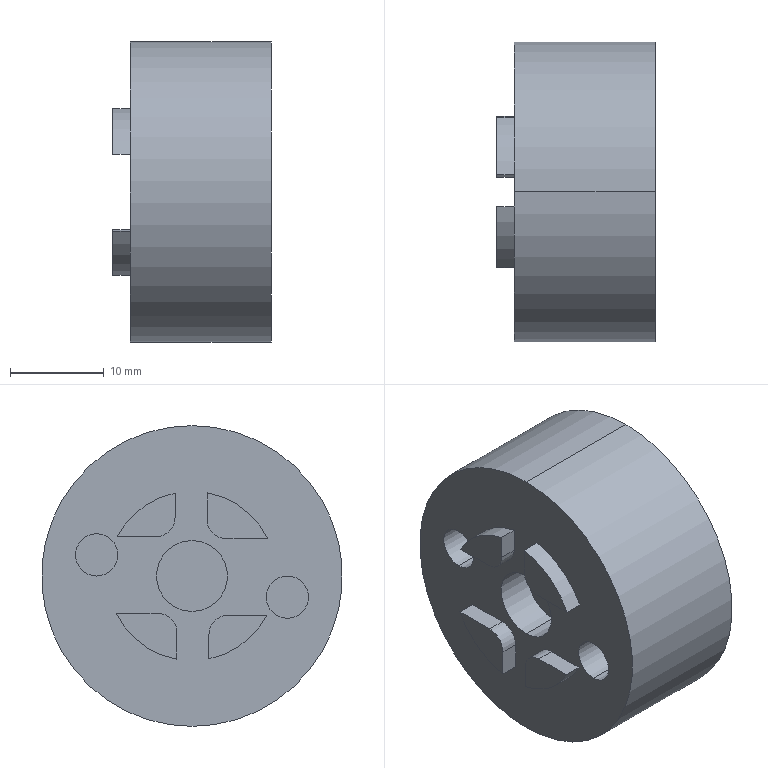Part | SolidWorks | features ICE 6, Cut 1, Extrusion 1, Fillet 1 | 1 solid | 38 faces | box 16.9 x 32 x 32 mm | volume 11867 mm3 | plane 22 | cylinder 16 | commonest cylinder face diameters 4 x4 4.5 x4 18 x4 7.55 x2 32 x2
STEP:
#1=CARTESIAN_POINT('',(3.5,-10.15,-4.5));
#2=VERTEX_POINT('',#1);
#3=CARTESIAN_POINT('',(3.5,-10.15,0.));
#4=VERTEX_POINT('',#3);
#5=CARTESIAN_POINT('',(3.5,-10.15,-2.25));
#6=DIRECTION('',(-1.,0.,0.));
#7=DIRECTION('',(0.,0.,1.));
#8=AXIS2_PLACEMENT_3D('',#5,#6,#7);
#9=CIRCLE('',#8,2.25);
#10=EDGE_CURVE('',#2,#4,#9,.T.);
#11=ORIENTED_EDGE('',*,*,#10,.F.);
#12=CARTESIAN_POINT('',(0.,-10.15,-4.5));
#13=VERTEX_POINT('',#12);
#14=CARTESIAN_POINT('',(3.5,-10.15,-4.5));
#15=DIRECTION('',(-1.,0.,0.));
#16=VECTOR('',#15,1000.);
#17=LINE('',#14,#16);
#18=EDGE_CURVE('',#2,#13,#17,.T.);
#19=ORIENTED_EDGE('',*,*,#18,.T.);
#20=CARTESIAN_POINT('',(0.,-10.15,0.));
#21=VERTEX_POINT('',#20);
#22=CARTESIAN_POINT('',(0.,-10.15,-2.25));
#23=DIRECTION('',(-1.,0.,0.));
#24=DIRECTION('',(0.,0.,1.));
#25=AXIS2_PLACEMENT_3D('',#22,#23,#24);
#26=CIRCLE('',#25,2.25);
#27=EDGE_CURVE('',#13,#21,#26,.T.);
#28=ORIENTED_EDGE('',*,*,#27,.T.);
#29=CARTESIAN_POINT('',(3.5,-10.15,0.));
#30=DIRECTION('',(-1.,0.,0.));
#31=VECTOR('',#30,1000.);
#32=LINE('',#29,#31);
#33=EDGE_CURVE('',#4,#21,#32,.T.);
#34=ORIENTED_EDGE('',*,*,#33,.F.);
#35=EDGE_LOOP('',(#11,#19,#28,#34));
#36=FACE_OUTER_BOUND('',#35,.T.);
#37=CARTESIAN_POINT('',(3.5,-10.15,-2.25));
#38=DIRECTION('',(-1.,0.,0.));
#39=DIRECTION('',(0.,0.,1.));
#40=AXIS2_PLACEMENT_3D('',#37,#38,#39);
#41=CYLINDRICAL_SURFACE('',#40,2.25);
#42=ADVANCED_FACE('',(#36),#41,.F.);
#43=CARTESIAN_POINT('',(3.5,10.15,0.));
#44=VERTEX_POINT('',#43);
#45=CARTESIAN_POINT('',(3.5,10.15,4.5));
#46=VERTEX_POINT('',#45);
#47=CARTESIAN_POINT('',(3.5,10.15,2.25));
#48=DIRECTION('',(-1.,0.,0.));
#49=DIRECTION('',(0.,0.,1.));
#50=AXIS2_PLACEMENT_3D('',#47,#48,#49);
#51=CIRCLE('',#50,2.25);
#52=EDGE_CURVE('',#44,#46,#51,.T.);
#53=ORIENTED_EDGE('',*,*,#52,.F.);
#54=CARTESIAN_POINT('',(0.,10.15,0.));
#55=VERTEX_POINT('',#54);
#56=CARTESIAN_POINT('',(3.5,10.15,0.));
#57=DIRECTION('',(-1.,0.,0.));
#58=VECTOR('',#57,1000.);
#59=LINE('',#56,#58);
#60=EDGE_CURVE('',#44,#55,#59,.T.);
#61=ORIENTED_EDGE('',*,*,#60,.T.);
#62=CARTESIAN_POINT('',(0.,10.15,4.5));
#63=VERTEX_POINT('',#62);
#64=CARTESIAN_POINT('',(0.,10.15,2.25));
#65=DIRECTION('',(-1.,0.,0.));
#66=DIRECTION('',(0.,0.,1.));
#67=AXIS2_PLACEMENT_3D('',#64,#65,#66);
#68=CIRCLE('',#67,2.25);
#69=EDGE_CURVE('',#55,#63,#68,.T.);
#70=ORIENTED_EDGE('',*,*,#69,.T.);
#71=CARTESIAN_POINT('',(3.5,10.15,4.5));
#72=DIRECTION('',(-1.,0.,0.));
#73=VECTOR('',#72,1000.);
#74=LINE('',#71,#73);
#75=EDGE_CURVE('',#46,#63,#74,.T.);
#76=ORIENTED_EDGE('',*,*,#75,.F.);
#77=EDGE_LOOP('',(#53,#61,#70,#76));
#78=FACE_OUTER_BOUND('',#77,.T.);
#79=CARTESIAN_POINT('',(3.5,10.15,2.25));
#80=DIRECTION('',(-1.,0.,0.));
#81=DIRECTION('',(0.,0.,1.));
#82=AXIS2_PLACEMENT_3D('',#79,#80,#81);
#83=CYLINDRICAL_SURFACE('',#82,2.25);
#84=ADVANCED_FACE('',(#78),#83,.F.);
#85=CARTESIAN_POINT('',(4.,0.,-3.775));
#86=VERTEX_POINT('',#85);
#87=CARTESIAN_POINT('',(4.,0.,3.775));
#88=VERTEX_POINT('',#87);
#89=CARTESIAN_POINT('',(4.,0.,0.));
#90=DIRECTION('',(-1.,0.,0.));
#91=DIRECTION('',(0.,0.,1.));
#92=AXIS2_PLACEMENT_3D('',#89,#90,#91);
#93=CIRCLE('',#92,3.775);
#94=EDGE_CURVE('',#86,#88,#93,.T.);
#95=ORIENTED_EDGE('',*,*,#94,.F.);
#96=CARTESIAN_POINT('',(0.,0.,-3.775));
#97=VERTEX_POINT('',#96);
#98=CARTESIAN_POINT('',(4.,0.,-3.775));
#99=DIRECTION('',(-1.,0.,0.));
#100=VECTOR('',#99,1000.);
#101=LINE('',#98,#100);
#102=EDGE_CURVE('',#86,#97,#101,.T.);
#103=ORIENTED_EDGE('',*,*,#102,.T.);
#104=CARTESIAN_POINT('',(0.,0.,3.775));
#105=VERTEX_POINT('',#104);
#106=CARTESIAN_POINT('',(0.,0.,0.));
#107=DIRECTION('',(-1.,0.,0.));
#108=DIRECTION('',(0.,0.,1.));
#109=AXIS2_PLACEMENT_3D('',#106,#107,#108);
#110=CIRCLE('',#109,3.775);
#111=EDGE_CURVE('',#97,#105,#110,.T.);
#112=ORIENTED_EDGE('',*,*,#111,.T.);
#113=CARTESIAN_POINT('',(4.,0.,3.775));
#114=DIRECTION('',(-1.,0.,0.));
#115=VECTOR('',#114,1000.);
#116=LINE('',#113,#115);
#117=EDGE_CURVE('',#88,#105,#116,.T.);
#118=ORIENTED_EDGE('',*,*,#117,.F.);
#119=EDGE_LOOP('',(#95,#103,#112,#118));
#120=FACE_OUTER_BOUND('',#119,.T.);
#121=CARTESIAN_POINT('',(4.,0.,0.));
#122=DIRECTION('',(-1.,0.,0.));
#123=DIRECTION('',(0.,0.,1.));
#124=AXIS2_PLACEMENT_3D('',#121,#122,#123);
#125=CYLINDRICAL_SURFACE('',#124,3.775);
#126=ADVANCED_FACE('',(#120),#125,.F.);
#127=CARTESIAN_POINT('',(15.,0.,-16.));
#128=VERTEX_POINT('',#127);
#129=CARTESIAN_POINT('',(15.,0.,16.));
#130=VERTEX_POINT('',#129);
#131=CARTESIAN_POINT('',(15.,0.,0.));
#132=DIRECTION('',(1.,0.,0.));
#133=DIRECTION('',(0.,0.,-1.));
#134=AXIS2_PLACEMENT_3D('',#131,#132,#133);
#135=CIRCLE('',#134,16.);
#136=EDGE_CURVE('',#128,#130,#135,.T.);
#137=ORIENTED_EDGE('',*,*,#136,.F.);
#138=CARTESIAN_POINT('',(0.,0.,-16.));
#139=VERTEX_POINT('',#138);
#140=CARTESIAN_POINT('',(15.,0.,-16.));
#141=DIRECTION('',(-1.,0.,0.));
#142=VECTOR('',#141,1000.);
#143=LINE('',#140,#142);
#144=EDGE_CURVE('',#128,#139,#143,.T.);
#145=ORIENTED_EDGE('',*,*,#144,.T.);
#146=CARTESIAN_POINT('',(0.,0.,16.));
#147=VERTEX_POINT('',#146);
#148=CARTESIAN_POINT('',(0.,0.,0.));
#149=DIRECTION('',(1.,0.,0.));
#150=DIRECTION('',(0.,0.,-1.));
#151=AXIS2_PLACEMENT_3D('',#148,#149,#150);
#152=CIRCLE('',#151,16.);
#153=EDGE_CURVE('',#139,#147,#152,.T.);
#154=ORIENTED_EDGE('',*,*,#153,.T.);
#155=CARTESIAN_POINT('',(15.,0.,16.));
#156=DIRECTION('',(-1.,0.,0.));
#157=VECTOR('',#156,1000.);
#158=LINE('',#155,#157);
#159=EDGE_CURVE('',#130,#147,#158,.T.);
#160=ORIENTED_EDGE('',*,*,#159,.F.);
#161=EDGE_LOOP('',(#137,#145,#154,#160));
#162=FACE_OUTER_BOUND('',#161,.T.);
#163=CARTESIAN_POINT('',(15.,0.,0.));
#164=DIRECTION('',(-1.,0.,0.));
#165=DIRECTION('',(0.,0.,1.));
#166=AXIS2_PLACEMENT_3D('',#163,#164,#165);
#167=CYLINDRICAL_SURFACE('',#166,16.);
#168=ADVANCED_FACE('',(#162),#167,.T.);
#169=CARTESIAN_POINT('',(0.,7.96,4.2));
#170=VERTEX_POINT('',#169);
#171=CARTESIAN_POINT('',(-1.9,7.96,4.2));
#172=VERTEX_POINT('',#171);
#173=CARTESIAN_POINT('',(49.994,7.96,4.2));
#174=DIRECTION('',(-1.,0.,0.));
#175=VECTOR('',#174,1000.);
#176=LINE('',#173,#175);
#177=EDGE_CURVE('',#170,#172,#176,.T.);
#178=ORIENTED_EDGE('',*,*,#177,.F.);
#179=CARTESIAN_POINT('',(0.,3.8,4.2));
#180=VERTEX_POINT('',#179);
#181=CARTESIAN_POINT('',(0.,17.12,4.2));
#182=DIRECTION('',(0.,-1.,0.));
#183=VECTOR('',#182,1000.);
#184=LINE('',#181,#183);
#185=EDGE_CURVE('',#170,#180,#184,.T.);
#186=ORIENTED_EDGE('',*,*,#185,.T.);
#187=CARTESIAN_POINT('',(-1.9,3.8,4.2));
#188=VERTEX_POINT('',#187);
#189=CARTESIAN_POINT('',(-1.9,3.8,4.2));
#190=DIRECTION('',(-1.,0.,0.));
#191=VECTOR('',#190,1000.);
#192=LINE('',#189,#191);
#193=EDGE_CURVE('',#180,#188,#192,.T.);
#194=ORIENTED_EDGE('',*,*,#193,.T.);
#195=CARTESIAN_POINT('',(-1.9,17.12,4.2));
#196=DIRECTION('',(0.,-1.,0.));
#197=VECTOR('',#196,1000.);
#198=LINE('',#195,#197);
#199=EDGE_CURVE('',#172,#188,#198,.T.);
#200=ORIENTED_EDGE('',*,*,#199,.F.);
#201=EDGE_LOOP('',(#178,#186,#194,#200));
#202=FACE_OUTER_BOUND('',#201,.T.);
#203=CARTESIAN_POINT('',(-1.9,17.12,4.2));
#204=DIRECTION('',(0.,0.,1.));
#205=DIRECTION('',(0.,-1.,0.));
#206=AXIS2_PLACEMENT_3D('',#203,#204,#205);
#207=PLANE('',#206);
#208=ADVANCED_FACE('',(#202),#207,.F.);
#209=CARTESIAN_POINT('',(-1.9,1.8,8.818));
#210=VERTEX_POINT('',#209);
#211=CARTESIAN_POINT('',(0.,1.8,8.818));
#212=VERTEX_POINT('',#211);
#213=CARTESIAN_POINT('',(49.994,1.8,8.818));
#214=DIRECTION('',(1.,0.,0.));
#215=VECTOR('',#214,1000.);
#216=LINE('',#213,#215);
#217=EDGE_CURVE('',#210,#212,#216,.T.);
#218=ORIENTED_EDGE('',*,*,#217,.F.);
#219=CARTESIAN_POINT('',(-1.9,1.8,6.2));
#220=VERTEX_POINT('',#219);
#221=CARTESIAN_POINT('',(-1.9,1.8,4.2));
#222=DIRECTION('',(0.,0.,1.));
#223=VECTOR('',#222,1000.);
#224=LINE('',#221,#223);
#225=EDGE_CURVE('',#220,#210,#224,.T.);
#226=ORIENTED_EDGE('',*,*,#225,.F.);
#227=CARTESIAN_POINT('',(0.,1.8,6.2));
#228=VERTEX_POINT('',#227);
#229=CARTESIAN_POINT('',(-1.9,1.8,6.2));
#230=DIRECTION('',(1.,0.,0.));
#231=VECTOR('',#230,1000.);
#232=LINE('',#229,#231);
#233=EDGE_CURVE('',#220,#228,#232,.T.);
#234=ORIENTED_EDGE('',*,*,#233,.T.);
#235=CARTESIAN_POINT('',(0.,1.8,4.2));
#236=DIRECTION('',(0.,0.,1.));
#237=VECTOR('',#236,1000.);
#238=LINE('',#235,#237);
#239=EDGE_CURVE('',#228,#212,#238,.T.);
#240=ORIENTED_EDGE('',*,*,#239,.T.);
#241=EDGE_LOOP('',(#218,#226,#234,#240));
#242=FACE_OUTER_BOUND('',#241,.T.);
#243=CARTESIAN_POINT('',(-1.9,1.8,4.2));
#244=DIRECTION('',(0.,1.,0.));
#245=DIRECTION('',(0.,0.,1.));
#246=AXIS2_PLACEMENT_3D('',#243,#244,#245);
#247=PLANE('',#246);
#248=ADVANCED_FACE('',(#242),#247,.F.);
#249=ORIENTED_EDGE('',*,*,#225,.T.);
#250=CARTESIAN_POINT('',(-1.9,0.,0.));
#251=DIRECTION('',(-1.,0.,0.));
#252=DIRECTION('',(0.,0.,1.));
#253=AXIS2_PLACEMENT_3D('',#250,#251,#252);
#254=CIRCLE('',#253,9.);
#255=EDGE_CURVE('',#210,#172,#254,.T.);
#256=ORIENTED_EDGE('',*,*,#255,.T.);
#257=ORIENTED_EDGE('',*,*,#199,.T.);
#258=CARTESIAN_POINT('',(-1.9,3.8,6.2));
#259=DIRECTION('',(-1.,0.,0.));
#260=DIRECTION('',(0.,0.,1.));
#261=AXIS2_PLACEMENT_3D('',#258,#259,#260);
#262=CIRCLE('',#261,2.);
#263=EDGE_CURVE('',#188,#220,#262,.T.);
#264=ORIENTED_EDGE('',*,*,#263,.T.);
#265=EDGE_LOOP('',(#249,#256,#257,#264));
#266=FACE_OUTER_BOUND('',#265,.T.);
#267=CARTESIAN_POINT('',(-1.9,0.,0.));
#268=DIRECTION('',(-1.,0.,0.));
#269=DIRECTION('',(0.,0.,1.));
#270=AXIS2_PLACEMENT_3D('',#267,#268,#269);
#271=PLANE('',#270);
#272=ADVANCED_FACE('',(#266),#271,.T.);
#273=CARTESIAN_POINT('',(0.,-7.96,-4.2));
#274=VERTEX_POINT('',#273);
#275=CARTESIAN_POINT('',(-1.9,-7.96,-4.2));
#276=VERTEX_POINT('',#275);
#277=CARTESIAN_POINT('',(49.994,-7.96,-4.2));
#278=DIRECTION('',(-1.,0.,0.));
#279=VECTOR('',#278,1000.);
#280=LINE('',#277,#279);
#281=EDGE_CURVE('',#274,#276,#280,.T.);
#282=ORIENTED_EDGE('',*,*,#281,.F.);
#283=CARTESIAN_POINT('',(0.,-3.8,-4.2));
#284=VERTEX_POINT('',#283);
#285=CARTESIAN_POINT('',(0.,-1.8,-4.2));
#286=DIRECTION('',(0.,1.,0.));
#287=VECTOR('',#286,1000.);
#288=LINE('',#285,#287);
#289=EDGE_CURVE('',#274,#284,#288,.T.);
#290=ORIENTED_EDGE('',*,*,#289,.T.);
#291=CARTESIAN_POINT('',(-1.9,-3.8,-4.2));
#292=VERTEX_POINT('',#291);
#293=CARTESIAN_POINT('',(-1.9,-3.8,-4.2));
#294=DIRECTION('',(-1.,0.,0.));
#295=VECTOR('',#294,1000.);
#296=LINE('',#293,#295);
#297=EDGE_CURVE('',#284,#292,#296,.T.);
#298=ORIENTED_EDGE('',*,*,#297,.T.);
#299=CARTESIAN_POINT('',(-1.9,-1.8,-4.2));
#300=DIRECTION('',(0.,1.,0.));
#301=VECTOR('',#300,1000.);
#302=LINE('',#299,#301);
#303=EDGE_CURVE('',#276,#292,#302,.T.);
#304=ORIENTED_EDGE('',*,*,#303,.F.);
#305=EDGE_LOOP('',(#282,#290,#298,#304));
#306=FACE_OUTER_BOUND('',#305,.T.);
#307=CARTESIAN_POINT('',(-1.9,-1.8,-4.2));
#308=DIRECTION('',(0.,0.,-1.));
#309=DIRECTION('',(-1.,0.,0.));
#310=AXIS2_PLACEMENT_3D('',#307,#308,#309);
#311=PLANE('',#310);
#312=ADVANCED_FACE('',(#306),#311,.F.);
#313=CARTESIAN_POINT('',(-1.9,-1.8,-8.818));
#314=VERTEX_POINT('',#313);
#315=CARTESIAN_POINT('',(0.,-1.8,-8.818));
#316=VERTEX_POINT('',#315);
#317=CARTESIAN_POINT('',(49.994,-1.8,-8.818));
#318=DIRECTION('',(1.,0.,0.));
#319=VECTOR('',#318,1000.);
#320=LINE('',#317,#319);
#321=EDGE_CURVE('',#314,#316,#320,.T.);
#322=ORIENTED_EDGE('',*,*,#321,.F.);
#323=CARTESIAN_POINT('',(-1.9,-1.8,-6.2));
#324=VERTEX_POINT('',#323);
#325=CARTESIAN_POINT('',(-1.9,-1.8,-20.455));
#326=DIRECTION('',(0.,0.,-1.));
#327=VECTOR('',#326,1000.);
#328=LINE('',#325,#327);
#329=EDGE_CURVE('',#324,#314,#328,.T.);
#330=ORIENTED_EDGE('',*,*,#329,.F.);
#331=CARTESIAN_POINT('',(0.,-1.8,-6.2));
#332=VERTEX_POINT('',#331);
#333=CARTESIAN_POINT('',(-1.9,-1.8,-6.2));
#334=DIRECTION('',(1.,0.,0.));
#335=VECTOR('',#334,1000.);
#336=LINE('',#333,#335);
#337=EDGE_CURVE('',#324,#332,#336,.T.);
#338=ORIENTED_EDGE('',*,*,#337,.T.);
#339=CARTESIAN_POINT('',(0.,-1.8,-20.455));
#340=DIRECTION('',(0.,0.,-1.));
#341=VECTOR('',#340,1000.);
#342=LINE('',#339,#341);
#343=EDGE_CURVE('',#332,#316,#342,.T.);
#344=ORIENTED_EDGE('',*,*,#343,.T.);
#345=EDGE_LOOP('',(#322,#330,#338,#344));
#346=FACE_OUTER_BOUND('',#345,.T.);
#347=CARTESIAN_POINT('',(-1.9,-1.8,-20.455));
#348=DIRECTION('',(0.,-1.,0.));
#349=DIRECTION('',(0.,0.,-1.));
#350=AXIS2_PLACEMENT_3D('',#347,#348,#349);
#351=PLANE('',#350);
#352=ADVANCED_FACE('',(#346),#351,.F.);
#353=ORIENTED_EDGE('',*,*,#329,.T.);
#354=CARTESIAN_POINT('',(-1.9,0.,0.));
#355=DIRECTION('',(-1.,0.,0.));
#356=DIRECTION('',(0.,0.,1.));
#357=AXIS2_PLACEMENT_3D('',#354,#355,#356);
#358=CIRCLE('',#357,9.);
#359=EDGE_CURVE('',#314,#276,#358,.T.);
#360=ORIENTED_EDGE('',*,*,#359,.T.);
#361=ORIENTED_EDGE('',*,*,#303,.T.);
#362=CARTESIAN_POINT('',(-1.9,-3.8,-6.2));
#363=DIRECTION('',(-1.,0.,0.));
#364=DIRECTION('',(0.,0.,1.));
#365=AXIS2_PLACEMENT_3D('',#362,#363,#364);
#366=CIRCLE('',#365,2.);
#367=EDGE_CURVE('',#292,#324,#366,.T.);
#368=ORIENTED_EDGE('',*,*,#367,.T.);
#369=EDGE_LOOP('',(#353,#360,#361,#368));
#370=FACE_OUTER_BOUND('',#369,.T.);
#371=CARTESIAN_POINT('',(-1.9,0.,0.));
#372=DIRECTION('',(-1.,0.,0.));
#373=DIRECTION('',(0.,0.,1.));
#374=AXIS2_PLACEMENT_3D('',#371,#372,#373);
#375=PLANE('',#374);
#376=ADVANCED_FACE('',(#370),#375,.T.);
#377=CARTESIAN_POINT('',(-1.9,8.062,-4.));
#378=VERTEX_POINT('',#377);
#379=CARTESIAN_POINT('',(0.,8.062,-4.));
#380=VERTEX_POINT('',#379);
#381=CARTESIAN_POINT('',(49.994,8.062,-4.));
#382=DIRECTION('',(1.,0.,0.));
#383=VECTOR('',#382,1000.);
#384=LINE('',#381,#383);
#385=EDGE_CURVE('',#378,#380,#384,.T.);
#386=ORIENTED_EDGE('',*,*,#385,.F.);
#387=CARTESIAN_POINT('',(-1.9,3.6,-4.));
#388=VERTEX_POINT('',#387);
#389=CARTESIAN_POINT('',(-1.9,1.6,-4.));
#390=DIRECTION('',(0.,1.,0.));
#391=VECTOR('',#390,1000.);
#392=LINE('',#389,#391);
#393=EDGE_CURVE('',#388,#378,#392,.T.);
#394=ORIENTED_EDGE('',*,*,#393,.F.);
#395=CARTESIAN_POINT('',(0.,3.6,-4.));
#396=VERTEX_POINT('',#395);
#397=CARTESIAN_POINT('',(-1.9,3.6,-4.));
#398=DIRECTION('',(1.,0.,0.));
#399=VECTOR('',#398,1000.);
#400=LINE('',#397,#399);
#401=EDGE_CURVE('',#388,#396,#400,.T.);
#402=ORIENTED_EDGE('',*,*,#401,.T.);
#403=CARTESIAN_POINT('',(0.,1.6,-4.));
#404=DIRECTION('',(0.,1.,0.));
#405=VECTOR('',#404,1000.);
#406=LINE('',#403,#405);
#407=EDGE_CURVE('',#396,#380,#406,.T.);
#408=ORIENTED_EDGE('',*,*,#407,.T.);
#409=EDGE_LOOP('',(#386,#394,#402,#408));
#410=FACE_OUTER_BOUND('',#409,.T.);
#411=CARTESIAN_POINT('',(-1.9,1.6,-4.));
#412=DIRECTION('',(0.,0.,-1.));
#413=DIRECTION('',(-1.,0.,0.));
#414=AXIS2_PLACEMENT_3D('',#411,#412,#413);
#415=PLANE('',#414);
#416=ADVANCED_FACE('',(#410),#415,.F.);
#417=CARTESIAN_POINT('',(0.,1.6,-8.857));
#418=VERTEX_POINT('',#417);
#419=CARTESIAN_POINT('',(-1.9,1.6,-8.857));
#420=VERTEX_POINT('',#419);
#421=CARTESIAN_POINT('',(49.994,1.6,-8.857));
#422=DIRECTION('',(-1.,0.,0.));
#423=VECTOR('',#422,1000.);
#424=LINE('',#421,#423);
#425=EDGE_CURVE('',#418,#420,#424,.T.);
#426=ORIENTED_EDGE('',*,*,#425,.F.);
#427=CARTESIAN_POINT('',(0.,1.6,-6.));
#428=VERTEX_POINT('',#427);
#429=CARTESIAN_POINT('',(0.,1.6,-15.92));
#430=DIRECTION('',(0.,0.,1.));
#431=VECTOR('',#430,1000.);
#432=LINE('',#429,#431);
#433=EDGE_CURVE('',#418,#428,#432,.T.);
#434=ORIENTED_EDGE('',*,*,#433,.T.);
#435=CARTESIAN_POINT('',(-1.9,1.6,-6.));
#436=VERTEX_POINT('',#435);
#437=CARTESIAN_POINT('',(-1.9,1.6,-6.));
#438=DIRECTION('',(-1.,0.,0.));
#439=VECTOR('',#438,1000.);
#440=LINE('',#437,#439);
#441=EDGE_CURVE('',#428,#436,#440,.T.);
#442=ORIENTED_EDGE('',*,*,#441,.T.);
#443=CARTESIAN_POINT('',(-1.9,1.6,-15.92));
#444=DIRECTION('',(0.,0.,1.));
#445=VECTOR('',#444,1000.);
#446=LINE('',#443,#445);
#447=EDGE_CURVE('',#420,#436,#446,.T.);
#448=ORIENTED_EDGE('',*,*,#447,.F.);
#449=EDGE_LOOP('',(#426,#434,#442,#448));
#450=FACE_OUTER_BOUND('',#449,.T.);
#451=CARTESIAN_POINT('',(-1.9,1.6,-15.92));
#452=DIRECTION('',(0.,1.,0.));
#453=DIRECTION('',(0.,0.,1.));
#454=AXIS2_PLACEMENT_3D('',#451,#452,#453);
#455=PLANE('',#454);
#456=ADVANCED_FACE('',(#450),#455,.F.);
#457=ORIENTED_EDGE('',*,*,#393,.T.);
#458=CARTESIAN_POINT('',(-1.9,0.,0.));
#459=DIRECTION('',(-1.,0.,0.));
#460=DIRECTION('',(0.,0.,1.));
#461=AXIS2_PLACEMENT_3D('',#458,#459,#460);
#462=CIRCLE('',#461,9.);
#463=EDGE_CURVE('',#378,#420,#462,.T.);
#464=ORIENTED_EDGE('',*,*,#463,.T.);
#465=ORIENTED_EDGE('',*,*,#447,.T.);
#466=CARTESIAN_POINT('',(-1.9,3.6,-6.));
#467=DIRECTION('',(-1.,0.,0.));
#468=DIRECTION('',(0.,0.,1.));
#469=AXIS2_PLACEMENT_3D('',#466,#467,#468);
#470=CIRCLE('',#469,2.);
#471=EDGE_CURVE('',#436,#388,#470,.T.);
#472=ORIENTED_EDGE('',*,*,#471,.T.);
#473=EDGE_LOOP('',(#457,#464,#465,#472));
#474=FACE_OUTER_BOUND('',#473,.T.);
#475=CARTESIAN_POINT('',(-1.9,0.,0.));
#476=DIRECTION('',(-1.,0.,0.));
#477=DIRECTION('',(0.,0.,1.));
#478=AXIS2_PLACEMENT_3D('',#475,#476,#477);
#479=PLANE('',#478);
#480=ADVANCED_FACE('',(#474),#479,.T.);
#481=CARTESIAN_POINT('',(0.,-1.6,8.857));
#482=VERTEX_POINT('',#481);
#483=CARTESIAN_POINT('',(-1.9,-1.6,8.857));
#484=VERTEX_POINT('',#483);
#485=CARTESIAN_POINT('',(49.994,-1.6,8.857));
#486=DIRECTION('',(-1.,0.,0.));
#487=VECTOR('',#486,1000.);
#488=LINE('',#485,#487);
#489=EDGE_CURVE('',#482,#484,#488,.T.);
#490=ORIENTED_EDGE('',*,*,#489,.F.);
#491=CARTESIAN_POINT('',(0.,-1.6,6.));
#492=VERTEX_POINT('',#491);
#493=CARTESIAN_POINT('',(0.,-1.6,4.));
#494=DIRECTION('',(0.,0.,-1.));
#495=VECTOR('',#494,1000.);
#496=LINE('',#493,#495);
#497=EDGE_CURVE('',#482,#492,#496,.T.);
#498=ORIENTED_EDGE('',*,*,#497,.T.);
#499=CARTESIAN_POINT('',(-1.9,-1.6,6.));
#500=VERTEX_POINT('',#499);
#501=CARTESIAN_POINT('',(-1.9,-1.6,6.));
#502=DIRECTION('',(-1.,0.,0.));
#503=VECTOR('',#502,1000.);
#504=LINE('',#501,#503);
#505=EDGE_CURVE('',#492,#500,#504,.T.);
#506=ORIENTED_EDGE('',*,*,#505,.T.);
#507=CARTESIAN_POINT('',(-1.9,-1.6,4.));
#508=DIRECTION('',(0.,0.,-1.));
#509=VECTOR('',#508,1000.);
#510=LINE('',#507,#509);
#511=EDGE_CURVE('',#484,#500,#510,.T.);
#512=ORIENTED_EDGE('',*,*,#511,.F.);
#513=EDGE_LOOP('',(#490,#498,#506,#512));
#514=FACE_OUTER_BOUND('',#513,.T.);
#515=CARTESIAN_POINT('',(-1.9,-1.6,4.));
#516=DIRECTION('',(0.,-1.,0.));
#517=DIRECTION('',(0.,0.,-1.));
#518=AXIS2_PLACEMENT_3D('',#515,#516,#517);
#519=PLANE('',#518);
#520=ADVANCED_FACE('',(#514),#519,.F.);
#521=CARTESIAN_POINT('',(-1.9,-8.062,4.));
#522=VERTEX_POINT('',#521);
#523=CARTESIAN_POINT('',(0.,-8.062,4.));
#524=VERTEX_POINT('',#523);
#525=CARTESIAN_POINT('',(49.994,-8.062,4.));
#526=DIRECTION('',(1.,0.,0.));
#527=VECTOR('',#526,1000.);
#528=LINE('',#525,#527);
#529=EDGE_CURVE('',#522,#524,#528,.T.);
#530=ORIENTED_EDGE('',*,*,#529,.F.);
#531=CARTESIAN_POINT('',(-1.9,-3.6,4.));
#532=VERTEX_POINT('',#531);
#533=CARTESIAN_POINT('',(-1.9,-15.492,4.));
#534=DIRECTION('',(0.,-1.,0.));
#535=VECTOR('',#534,1000.);
#536=LINE('',#533,#535);
#537=EDGE_CURVE('',#532,#522,#536,.T.);
#538=ORIENTED_EDGE('',*,*,#537,.F.);
#539=CARTESIAN_POINT('',(0.,-3.6,4.));
#540=VERTEX_POINT('',#539);
#541=CARTESIAN_POINT('',(-1.9,-3.6,4.));
#542=DIRECTION('',(1.,0.,0.));
#543=VECTOR('',#542,1000.);
#544=LINE('',#541,#543);
#545=EDGE_CURVE('',#532,#540,#544,.T.);
#546=ORIENTED_EDGE('',*,*,#545,.T.);
#547=CARTESIAN_POINT('',(0.,-15.492,4.));
#548=DIRECTION('',(0.,-1.,0.));
#549=VECTOR('',#548,1000.);
#550=LINE('',#547,#549);
#551=EDGE_CURVE('',#540,#524,#550,.T.);
#552=ORIENTED_EDGE('',*,*,#551,.T.);
#553=EDGE_LOOP('',(#530,#538,#546,#552));
#554=FACE_OUTER_BOUND('',#553,.T.);
#555=CARTESIAN_POINT('',(-1.9,-15.492,4.));
#556=DIRECTION('',(0.,0.,1.));
#557=DIRECTION('',(1.,0.,0.));
#558=AXIS2_PLACEMENT_3D('',#555,#556,#557);
#559=PLANE('',#558);
#560=ADVANCED_FACE('',(#554),#559,.F.);
#561=ORIENTED_EDGE('',*,*,#537,.T.);
#562=CARTESIAN_POINT('',(-1.9,0.,0.));
#563=DIRECTION('',(-1.,0.,0.));
#564=DIRECTION('',(0.,0.,1.));
#565=AXIS2_PLACEMENT_3D('',#562,#563,#564);
#566=CIRCLE('',#565,9.);
#567=EDGE_CURVE('',#522,#484,#566,.T.);
#568=ORIENTED_EDGE('',*,*,#567,.T.);
#569=ORIENTED_EDGE('',*,*,#511,.T.);
#570=CARTESIAN_POINT('',(-1.9,-3.6,6.));
#571=DIRECTION('',(-1.,0.,0.));
#572=DIRECTION('',(0.,0.,1.));
#573=AXIS2_PLACEMENT_3D('',#570,#571,#572);
#574=CIRCLE('',#573,2.);
#575=EDGE_CURVE('',#500,#532,#574,.T.);
#576=ORIENTED_EDGE('',*,*,#575,.T.);
#577=EDGE_LOOP('',(#561,#568,#569,#576));
#578=FACE_OUTER_BOUND('',#577,.T.);
#579=CARTESIAN_POINT('',(-1.9,0.,0.));
#580=DIRECTION('',(-1.,0.,0.));
#581=DIRECTION('',(0.,0.,1.));
#582=AXIS2_PLACEMENT_3D('',#579,#580,#581);
#583=PLANE('',#582);
#584=ADVANCED_FACE('',(#578),#583,.T.);
#585=CARTESIAN_POINT('',(0.,-10.15,-2.25));
#586=DIRECTION('',(-1.,0.,0.));
#587=DIRECTION('',(0.,0.,1.));
#588=AXIS2_PLACEMENT_3D('',#585,#586,#587);
#589=CIRCLE('',#588,2.25);
#590=EDGE_CURVE('',#21,#13,#589,.T.);
#591=ORIENTED_EDGE('',*,*,#590,.F.);
#592=ORIENTED_EDGE('',*,*,#27,.F.);
#593=EDGE_LOOP('',(#591,#592));
#594=FACE_BOUND('',#593,.T.);
#595=CARTESIAN_POINT('',(0.,10.15,2.25));
#596=DIRECTION('',(-1.,0.,0.));
#597=DIRECTION('',(0.,0.,1.));
#598=AXIS2_PLACEMENT_3D('',#595,#596,#597);
#599=CIRCLE('',#598,2.25);
#600=EDGE_CURVE('',#63,#55,#599,.T.);
#601=ORIENTED_EDGE('',*,*,#600,.F.);
#602=ORIENTED_EDGE('',*,*,#69,.F.);
#603=EDGE_LOOP('',(#601,#602));
#604=FACE_BOUND('',#603,.T.);
#605=ORIENTED_EDGE('',*,*,#185,.F.);
#606=CARTESIAN_POINT('',(0.,0.,0.));
#607=DIRECTION('',(-1.,0.,0.));
#608=DIRECTION('',(0.,0.,-1.));
#609=AXIS2_PLACEMENT_3D('',#606,#607,#608);
#610=CIRCLE('',#609,9.);
#611=EDGE_CURVE('',#212,#170,#610,.T.);
#612=ORIENTED_EDGE('',*,*,#611,.F.);
#613=ORIENTED_EDGE('',*,*,#239,.F.);
#614=CARTESIAN_POINT('',(0.,3.8,6.2));
#615=DIRECTION('',(1.,0.,0.));
#616=DIRECTION('',(0.,0.,-1.));
#617=AXIS2_PLACEMENT_3D('',#614,#615,#616);
#618=CIRCLE('',#617,2.);
#619=EDGE_CURVE('',#228,#180,#618,.T.);
#620=ORIENTED_EDGE('',*,*,#619,.T.);
#621=EDGE_LOOP('',(#605,#612,#613,#620));
#622=FACE_BOUND('',#621,.T.);
#623=ORIENTED_EDGE('',*,*,#289,.F.);
#624=CARTESIAN_POINT('',(0.,0.,0.));
#625=DIRECTION('',(-1.,0.,0.));
#626=DIRECTION('',(0.,0.,-1.));
#627=AXIS2_PLACEMENT_3D('',#624,#625,#626);
#628=CIRCLE('',#627,9.);
#629=EDGE_CURVE('',#316,#274,#628,.T.);
#630=ORIENTED_EDGE('',*,*,#629,.F.);
#631=ORIENTED_EDGE('',*,*,#343,.F.);
#632=CARTESIAN_POINT('',(0.,-3.8,-6.2));
#633=DIRECTION('',(1.,0.,0.));
#634=DIRECTION('',(0.,0.,-1.));
#635=AXIS2_PLACEMENT_3D('',#632,#633,#634);
#636=CIRCLE('',#635,2.);
#637=EDGE_CURVE('',#332,#284,#636,.T.);
#638=ORIENTED_EDGE('',*,*,#637,.T.);
#639=EDGE_LOOP('',(#623,#630,#631,#638));
#640=FACE_BOUND('',#639,.T.);
#641=CARTESIAN_POINT('',(0.,0.,0.));
#642=DIRECTION('',(1.,0.,0.));
#643=DIRECTION('',(0.,0.,-1.));
#644=AXIS2_PLACEMENT_3D('',#641,#642,#643);
#645=CIRCLE('',#644,16.);
#646=EDGE_CURVE('',#147,#139,#645,.T.);
#647=ORIENTED_EDGE('',*,*,#646,.F.);
#648=ORIENTED_EDGE('',*,*,#153,.F.);
#649=EDGE_LOOP('',(#647,#648));
#650=FACE_OUTER_BOUND('',#649,.T.);
#651=ORIENTED_EDGE('',*,*,#497,.F.);
#652=CARTESIAN_POINT('',(0.,0.,0.));
#653=DIRECTION('',(-1.,0.,0.));
#654=DIRECTION('',(0.,0.,-1.));
#655=AXIS2_PLACEMENT_3D('',#652,#653,#654);
#656=CIRCLE('',#655,9.);
#657=EDGE_CURVE('',#524,#482,#656,.T.);
#658=ORIENTED_EDGE('',*,*,#657,.F.);
#659=ORIENTED_EDGE('',*,*,#551,.F.);
#660=CARTESIAN_POINT('',(0.,-3.6,6.));
#661=DIRECTION('',(1.,0.,0.));
#662=DIRECTION('',(0.,0.,-1.));
#663=AXIS2_PLACEMENT_3D('',#660,#661,#662);
#664=CIRCLE('',#663,2.);
#665=EDGE_CURVE('',#540,#492,#664,.T.);
#666=ORIENTED_EDGE('',*,*,#665,.T.);
#667=EDGE_LOOP('',(#651,#658,#659,#666));
#668=FACE_BOUND('',#667,.T.);
#669=CARTESIAN_POINT('',(0.,0.,0.));
#670=DIRECTION('',(-1.,0.,0.));
#671=DIRECTION('',(0.,0.,-1.));
#672=AXIS2_PLACEMENT_3D('',#669,#670,#671);
#673=CIRCLE('',#672,9.);
#674=EDGE_CURVE('',#380,#418,#673,.T.);
#675=ORIENTED_EDGE('',*,*,#674,.F.);
#676=ORIENTED_EDGE('',*,*,#407,.F.);
#677=CARTESIAN_POINT('',(0.,3.6,-6.));
#678=DIRECTION('',(1.,0.,0.));
#679=DIRECTION('',(0.,0.,-1.));
#680=AXIS2_PLACEMENT_3D('',#677,#678,#679);
#681=CIRCLE('',#680,2.);
#682=EDGE_CURVE('',#396,#428,#681,.T.);
#683=ORIENTED_EDGE('',*,*,#682,.T.);
#684=ORIENTED_EDGE('',*,*,#433,.F.);
#685=EDGE_LOOP('',(#675,#676,#683,#684));
#686=FACE_BOUND('',#685,.T.);
#687=CARTESIAN_POINT('',(0.,0.,0.));
#688=DIRECTION('',(-1.,0.,0.));
#689=DIRECTION('',(0.,0.,1.));
#690=AXIS2_PLACEMENT_3D('',#687,#688,#689);
#691=CIRCLE('',#690,3.775);
#692=EDGE_CURVE('',#105,#97,#691,.T.);
#693=ORIENTED_EDGE('',*,*,#692,.F.);
#694=ORIENTED_EDGE('',*,*,#111,.F.);
#695=EDGE_LOOP('',(#693,#694));
#696=FACE_BOUND('',#695,.T.);
#697=CARTESIAN_POINT('',(0.,0.,0.));
#698=DIRECTION('',(1.,0.,0.));
#699=DIRECTION('',(0.,0.,-1.));
#700=AXIS2_PLACEMENT_3D('',#697,#698,#699);
#701=PLANE('',#700);
#702=ADVANCED_FACE('',(#594,#604,#622,#640,#650,#668,#686,#696),#701,.F.);
#703=ORIENTED_EDGE('',*,*,#144,.F.);
#704=CARTESIAN_POINT('',(15.,0.,0.));
#705=DIRECTION('',(1.,0.,0.));
#706=DIRECTION('',(0.,0.,-1.));
#707=AXIS2_PLACEMENT_3D('',#704,#705,#706);
#708=CIRCLE('',#707,16.);
#709=EDGE_CURVE('',#130,#128,#708,.T.);
#710=ORIENTED_EDGE('',*,*,#709,.F.);
#711=ORIENTED_EDGE('',*,*,#159,.T.);
#712=ORIENTED_EDGE('',*,*,#646,.T.);
#713=EDGE_LOOP('',(#703,#710,#711,#712));
#714=FACE_OUTER_BOUND('',#713,.T.);
#715=CARTESIAN_POINT('',(15.,0.,0.));
#716=DIRECTION('',(-1.,0.,0.));
#717=DIRECTION('',(0.,0.,1.));
#718=AXIS2_PLACEMENT_3D('',#715,#716,#717);
#719=CYLINDRICAL_SURFACE('',#718,16.);
#720=ADVANCED_FACE('',(#714),#719,.T.);
#721=CARTESIAN_POINT('',(15.,-2.5,-2.5));
#722=VERTEX_POINT('',#721);
#723=CARTESIAN_POINT('',(15.,2.5,-2.5));
#724=VERTEX_POINT('',#723);
#725=CARTESIAN_POINT('',(15.,2.5,-2.5));
#726=DIRECTION('',(0.,1.,0.));
#727=VECTOR('',#726,1000.);
#728=LINE('',#725,#727);
#729=EDGE_CURVE('',#722,#724,#728,.T.);
#730=ORIENTED_EDGE('',*,*,#729,.F.);
#731=CARTESIAN_POINT('',(15.,-2.5,2.5));
#732=VERTEX_POINT('',#731);
#733=CARTESIAN_POINT('',(15.,-2.5,2.5));
#734=DIRECTION('',(0.,0.,-1.));
#735=VECTOR('',#734,1000.);
#736=LINE('',#733,#735);
#737=EDGE_CURVE('',#732,#722,#736,.T.);
#738=ORIENTED_EDGE('',*,*,#737,.F.);
#739=CARTESIAN_POINT('',(15.,2.5,2.5));
#740=VERTEX_POINT('',#739);
#741=CARTESIAN_POINT('',(15.,2.5,2.5));
#742=DIRECTION('',(0.,-1.,0.));
#743=VECTOR('',#742,1000.);
#744=LINE('',#741,#743);
#745=EDGE_CURVE('',#740,#732,#744,.T.);
#746=ORIENTED_EDGE('',*,*,#745,.F.);
#747=CARTESIAN_POINT('',(15.,2.5,2.5));
#748=DIRECTION('',(0.,0.,1.));
#749=VECTOR('',#748,1000.);
#750=LINE('',#747,#749);
#751=EDGE_CURVE('',#724,#740,#750,.T.);
#752=ORIENTED_EDGE('',*,*,#751,.F.);
#753=EDGE_LOOP('',(#730,#738,#746,#752));
#754=FACE_BOUND('',#753,.T.);
#755=ORIENTED_EDGE('',*,*,#709,.T.);
#756=ORIENTED_EDGE('',*,*,#136,.T.);
#757=EDGE_LOOP('',(#755,#756));
#758=FACE_OUTER_BOUND('',#757,.T.);
#759=CARTESIAN_POINT('',(15.,0.,0.));
#760=DIRECTION('',(1.,0.,0.));
#761=DIRECTION('',(0.,0.,-1.));
#762=AXIS2_PLACEMENT_3D('',#759,#760,#761);
#763=PLANE('',#762);
#764=ADVANCED_FACE('',(#754,#758),#763,.T.);
#765=ORIENTED_EDGE('',*,*,#102,.F.);
#766=CARTESIAN_POINT('',(4.,0.,0.));
#767=DIRECTION('',(-1.,0.,0.));
#768=DIRECTION('',(0.,0.,1.));
#769=AXIS2_PLACEMENT_3D('',#766,#767,#768);
#770=CIRCLE('',#769,3.775);
#771=EDGE_CURVE('',#88,#86,#770,.T.);
#772=ORIENTED_EDGE('',*,*,#771,.F.);
#773=ORIENTED_EDGE('',*,*,#117,.T.);
#774=ORIENTED_EDGE('',*,*,#692,.T.);
#775=EDGE_LOOP('',(#765,#772,#773,#774));
#776=FACE_OUTER_BOUND('',#775,.T.);
#777=CARTESIAN_POINT('',(4.,0.,0.));
#778=DIRECTION('',(-1.,0.,0.));
#779=DIRECTION('',(0.,0.,1.));
#780=AXIS2_PLACEMENT_3D('',#777,#778,#779);
#781=CYLINDRICAL_SURFACE('',#780,3.775);
#782=ADVANCED_FACE('',(#776),#781,.F.);
#783=ORIENTED_EDGE('',*,*,#771,.T.);
#784=ORIENTED_EDGE('',*,*,#94,.T.);
#785=EDGE_LOOP('',(#783,#784));
#786=FACE_OUTER_BOUND('',#785,.T.);
#787=CARTESIAN_POINT('',(4.,0.,0.));
#788=DIRECTION('',(-1.,0.,0.));
#789=DIRECTION('',(0.,0.,1.));
#790=AXIS2_PLACEMENT_3D('',#787,#788,#789);
#791=PLANE('',#790);
#792=ADVANCED_FACE('',(#786),#791,.T.);
#793=ORIENTED_EDGE('',*,*,#60,.F.);
#794=CARTESIAN_POINT('',(3.5,10.15,2.25));
#795=DIRECTION('',(-1.,0.,0.));
#796=DIRECTION('',(0.,0.,1.));
#797=AXIS2_PLACEMENT_3D('',#794,#795,#796);
#798=CIRCLE('',#797,2.25);
#799=EDGE_CURVE('',#46,#44,#798,.T.);
#800=ORIENTED_EDGE('',*,*,#799,.F.);
#801=ORIENTED_EDGE('',*,*,#75,.T.);
#802=ORIENTED_EDGE('',*,*,#600,.T.);
#803=EDGE_LOOP('',(#793,#800,#801,#802));
#804=FACE_OUTER_BOUND('',#803,.T.);
#805=CARTESIAN_POINT('',(3.5,10.15,2.25));
#806=DIRECTION('',(-1.,0.,0.));
#807=DIRECTION('',(0.,0.,1.));
#808=AXIS2_PLACEMENT_3D('',#805,#806,#807);
#809=CYLINDRICAL_SURFACE('',#808,2.25);
#810=ADVANCED_FACE('',(#804),#809,.F.);
#811=ORIENTED_EDGE('',*,*,#799,.T.);
#812=ORIENTED_EDGE('',*,*,#52,.T.);
#813=EDGE_LOOP('',(#811,#812));
#814=FACE_OUTER_BOUND('',#813,.T.);
#815=CARTESIAN_POINT('',(3.5,10.15,2.25));
#816=DIRECTION('',(-1.,0.,0.));
#817=DIRECTION('',(0.,0.,1.));
#818=AXIS2_PLACEMENT_3D('',#815,#816,#817);
#819=PLANE('',#818);
#820=ADVANCED_FACE('',(#814),#819,.T.);
#821=ORIENTED_EDGE('',*,*,#18,.F.);
#822=CARTESIAN_POINT('',(3.5,-10.15,-2.25));
#823=DIRECTION('',(-1.,0.,0.));
#824=DIRECTION('',(0.,0.,1.));
#825=AXIS2_PLACEMENT_3D('',#822,#823,#824);
#826=CIRCLE('',#825,2.25);
#827=EDGE_CURVE('',#4,#2,#826,.T.);
#828=ORIENTED_EDGE('',*,*,#827,.F.);
#829=ORIENTED_EDGE('',*,*,#33,.T.);
#830=ORIENTED_EDGE('',*,*,#590,.T.);
#831=EDGE_LOOP('',(#821,#828,#829,#830));
#832=FACE_OUTER_BOUND('',#831,.T.);
#833=CARTESIAN_POINT('',(3.5,-10.15,-2.25));
#834=DIRECTION('',(-1.,0.,0.));
#835=DIRECTION('',(0.,0.,1.));
#836=AXIS2_PLACEMENT_3D('',#833,#834,#835);
#837=CYLINDRICAL_SURFACE('',#836,2.25);
#838=ADVANCED_FACE('',(#832),#837,.F.);
#839=ORIENTED_EDGE('',*,*,#827,.T.);
#840=ORIENTED_EDGE('',*,*,#10,.T.);
#841=EDGE_LOOP('',(#839,#840));
#842=FACE_OUTER_BOUND('',#841,.T.);
#843=CARTESIAN_POINT('',(3.5,-10.15,-2.25));
#844=DIRECTION('',(-1.,0.,0.));
#845=DIRECTION('',(0.,0.,1.));
#846=AXIS2_PLACEMENT_3D('',#843,#844,#845);
#847=PLANE('',#846);
#848=ADVANCED_FACE('',(#842),#847,.T.);
#849=ORIENTED_EDGE('',*,*,#367,.F.);
#850=ORIENTED_EDGE('',*,*,#297,.F.);
#851=ORIENTED_EDGE('',*,*,#637,.F.);
#852=ORIENTED_EDGE('',*,*,#337,.F.);
#853=EDGE_LOOP('',(#849,#850,#851,#852));
#854=FACE_OUTER_BOUND('',#853,.T.);
#855=CARTESIAN_POINT('',(-1.9,-3.8,-6.2));
#856=DIRECTION('',(1.,0.,0.));
#857=DIRECTION('',(0.,0.,-1.));
#858=AXIS2_PLACEMENT_3D('',#855,#856,#857);
#859=CYLINDRICAL_SURFACE('',#858,2.);
#860=ADVANCED_FACE('',(#854),#859,.T.);
#861=ORIENTED_EDGE('',*,*,#263,.F.);
#862=ORIENTED_EDGE('',*,*,#193,.F.);
#863=ORIENTED_EDGE('',*,*,#619,.F.);
#864=ORIENTED_EDGE('',*,*,#233,.F.);
#865=EDGE_LOOP('',(#861,#862,#863,#864));
#866=FACE_OUTER_BOUND('',#865,.T.);
#867=CARTESIAN_POINT('',(-1.9,3.8,6.2));
#868=DIRECTION('',(1.,0.,0.));
#869=DIRECTION('',(0.,0.,-1.));
#870=AXIS2_PLACEMENT_3D('',#867,#868,#869);
#871=CYLINDRICAL_SURFACE('',#870,2.);
#872=ADVANCED_FACE('',(#866),#871,.T.);
#873=ORIENTED_EDGE('',*,*,#471,.F.);
#874=ORIENTED_EDGE('',*,*,#441,.F.);
#875=ORIENTED_EDGE('',*,*,#682,.F.);
#876=ORIENTED_EDGE('',*,*,#401,.F.);
#877=EDGE_LOOP('',(#873,#874,#875,#876));
#878=FACE_OUTER_BOUND('',#877,.T.);
#879=CARTESIAN_POINT('',(-1.9,3.6,-6.));
#880=DIRECTION('',(1.,0.,0.));
#881=DIRECTION('',(0.,0.,-1.));
#882=AXIS2_PLACEMENT_3D('',#879,#880,#881);
#883=CYLINDRICAL_SURFACE('',#882,2.);
#884=ADVANCED_FACE('',(#878),#883,.T.);
#885=ORIENTED_EDGE('',*,*,#575,.F.);
#886=ORIENTED_EDGE('',*,*,#505,.F.);
#887=ORIENTED_EDGE('',*,*,#665,.F.);
#888=ORIENTED_EDGE('',*,*,#545,.F.);
#889=EDGE_LOOP('',(#885,#886,#887,#888));
#890=FACE_OUTER_BOUND('',#889,.T.);
#891=CARTESIAN_POINT('',(-1.9,-3.6,6.));
#892=DIRECTION('',(1.,0.,0.));
#893=DIRECTION('',(0.,0.,-1.));
#894=AXIS2_PLACEMENT_3D('',#891,#892,#893);
#895=CYLINDRICAL_SURFACE('',#894,2.);
#896=ADVANCED_FACE('',(#890),#895,.T.);
#897=ORIENTED_EDGE('',*,*,#489,.T.);
#898=ORIENTED_EDGE('',*,*,#567,.F.);
#899=ORIENTED_EDGE('',*,*,#529,.T.);
#900=ORIENTED_EDGE('',*,*,#657,.T.);
#901=EDGE_LOOP('',(#897,#898,#899,#900));
#902=FACE_OUTER_BOUND('',#901,.T.);
#903=CARTESIAN_POINT('',(49.994,0.,0.));
#904=DIRECTION('',(-1.,0.,0.));
#905=DIRECTION('',(0.,0.,1.));
#906=AXIS2_PLACEMENT_3D('',#903,#904,#905);
#907=CYLINDRICAL_SURFACE('',#906,9.);
#908=ADVANCED_FACE('',(#902),#907,.T.);
#909=ORIENTED_EDGE('',*,*,#385,.T.);
#910=ORIENTED_EDGE('',*,*,#674,.T.);
#911=ORIENTED_EDGE('',*,*,#425,.T.);
#912=ORIENTED_EDGE('',*,*,#463,.F.);
#913=EDGE_LOOP('',(#909,#910,#911,#912));
#914=FACE_OUTER_BOUND('',#913,.T.);
#915=CARTESIAN_POINT('',(49.994,0.,0.));
#916=DIRECTION('',(-1.,0.,0.));
#917=DIRECTION('',(0.,0.,1.));
#918=AXIS2_PLACEMENT_3D('',#915,#916,#917);
#919=CYLINDRICAL_SURFACE('',#918,9.);
#920=ADVANCED_FACE('',(#914),#919,.T.);
#921=ORIENTED_EDGE('',*,*,#281,.T.);
#922=ORIENTED_EDGE('',*,*,#359,.F.);
#923=ORIENTED_EDGE('',*,*,#321,.T.);
#924=ORIENTED_EDGE('',*,*,#629,.T.);
#925=EDGE_LOOP('',(#921,#922,#923,#924));
#926=FACE_OUTER_BOUND('',#925,.T.);
#927=CARTESIAN_POINT('',(49.994,0.,0.));
#928=DIRECTION('',(-1.,0.,0.));
#929=DIRECTION('',(0.,0.,1.));
#930=AXIS2_PLACEMENT_3D('',#927,#928,#929);
#931=CYLINDRICAL_SURFACE('',#930,9.);
#932=ADVANCED_FACE('',(#926),#931,.T.);
#933=ORIENTED_EDGE('',*,*,#177,.T.);
#934=ORIENTED_EDGE('',*,*,#255,.F.);
#935=ORIENTED_EDGE('',*,*,#217,.T.);
#936=ORIENTED_EDGE('',*,*,#611,.T.);
#937=EDGE_LOOP('',(#933,#934,#935,#936));
#938=FACE_OUTER_BOUND('',#937,.T.);
#939=CARTESIAN_POINT('',(49.994,0.,0.));
#940=DIRECTION('',(-1.,0.,0.));
#941=DIRECTION('',(0.,0.,1.));
#942=AXIS2_PLACEMENT_3D('',#939,#940,#941);
#943=CYLINDRICAL_SURFACE('',#942,9.);
#944=ADVANCED_FACE('',(#938),#943,.T.);
#945=ORIENTED_EDGE('',*,*,#729,.T.);
#946=CARTESIAN_POINT('',(13.,2.5,-2.5));
#947=VERTEX_POINT('',#946);
#948=CARTESIAN_POINT('',(13.,2.5,-2.5));
#949=DIRECTION('',(1.,0.,0.));
#950=VECTOR('',#949,1000.);
#951=LINE('',#948,#950);
#952=EDGE_CURVE('',#947,#724,#951,.T.);
#953=ORIENTED_EDGE('',*,*,#952,.F.);
#954=CARTESIAN_POINT('',(13.,-2.5,-2.5));
#955=VERTEX_POINT('',#954);
#956=CARTESIAN_POINT('',(13.,2.5,-2.5));
#957=DIRECTION('',(0.,1.,0.));
#958=VECTOR('',#957,1000.);
#959=LINE('',#956,#958);
#960=EDGE_CURVE('',#955,#947,#959,.T.);
#961=ORIENTED_EDGE('',*,*,#960,.F.);
#962=CARTESIAN_POINT('',(13.,-2.5,-2.5));
#963=DIRECTION('',(1.,0.,0.));
#964=VECTOR('',#963,1000.);
#965=LINE('',#962,#964);
#966=EDGE_CURVE('',#955,#722,#965,.T.);
#967=ORIENTED_EDGE('',*,*,#966,.T.);
#968=EDGE_LOOP('',(#945,#953,#961,#967));
#969=FACE_OUTER_BOUND('',#968,.T.);
#970=CARTESIAN_POINT('',(13.,2.5,-2.5));
#971=DIRECTION('',(0.,0.,-1.));
#972=DIRECTION('',(-1.,0.,0.));
#973=AXIS2_PLACEMENT_3D('',#970,#971,#972);
#974=PLANE('',#973);
#975=ADVANCED_FACE('',(#969),#974,.F.);
#976=ORIENTED_EDGE('',*,*,#737,.T.);
#977=ORIENTED_EDGE('',*,*,#966,.F.);
#978=CARTESIAN_POINT('',(13.,-2.5,2.5));
#979=VERTEX_POINT('',#978);
#980=CARTESIAN_POINT('',(13.,-2.5,2.5));
#981=DIRECTION('',(0.,0.,-1.));
#982=VECTOR('',#981,1000.);
#983=LINE('',#980,#982);
#984=EDGE_CURVE('',#979,#955,#983,.T.);
#985=ORIENTED_EDGE('',*,*,#984,.F.);
#986=CARTESIAN_POINT('',(13.,-2.5,2.5));
#987=DIRECTION('',(1.,0.,0.));
#988=VECTOR('',#987,1000.);
#989=LINE('',#986,#988);
#990=EDGE_CURVE('',#979,#732,#989,.T.);
#991=ORIENTED_EDGE('',*,*,#990,.T.);
#992=EDGE_LOOP('',(#976,#977,#985,#991));
#993=FACE_OUTER_BOUND('',#992,.T.);
#994=CARTESIAN_POINT('',(13.,-2.5,2.5));
#995=DIRECTION('',(0.,-1.,0.));
#996=DIRECTION('',(0.,0.,-1.));
#997=AXIS2_PLACEMENT_3D('',#994,#995,#996);
#998=PLANE('',#997);
#999=ADVANCED_FACE('',(#993),#998,.F.);
#1000=ORIENTED_EDGE('',*,*,#745,.T.);
#1001=ORIENTED_EDGE('',*,*,#990,.F.);
#1002=CARTESIAN_POINT('',(13.,2.5,2.5));
#1003=VERTEX_POINT('',#1002);
#1004=CARTESIAN_POINT('',(13.,2.5,2.5));
#1005=DIRECTION('',(0.,-1.,0.));
#1006=VECTOR('',#1005,1000.);
#1007=LINE('',#1004,#1006);
#1008=EDGE_CURVE('',#1003,#979,#1007,.T.);
#1009=ORIENTED_EDGE('',*,*,#1008,.F.);
#1010=CARTESIAN_POINT('',(13.,2.5,2.5));
#1011=DIRECTION('',(1.,0.,0.));
#1012=VECTOR('',#1011,1000.);
#1013=LINE('',#1010,#1012);
#1014=EDGE_CURVE('',#1003,#740,#1013,.T.);
#1015=ORIENTED_EDGE('',*,*,#1014,.T.);
#1016=EDGE_LOOP('',(#1000,#1001,#1009,#1015));
#1017=FACE_OUTER_BOUND('',#1016,.T.);
#1018=CARTESIAN_POINT('',(13.,2.5,2.5));
#1019=DIRECTION('',(0.,0.,1.));
#1020=DIRECTION('',(0.,-1.,0.));
#1021=AXIS2_PLACEMENT_3D('',#1018,#1019,#1020);
#1022=PLANE('',#1021);
#1023=ADVANCED_FACE('',(#1017),#1022,.F.);
#1024=ORIENTED_EDGE('',*,*,#751,.T.);
#1025=ORIENTED_EDGE('',*,*,#1014,.F.);
#1026=CARTESIAN_POINT('',(13.,2.5,2.5));
#1027=DIRECTION('',(0.,0.,1.));
#1028=VECTOR('',#1027,1000.);
#1029=LINE('',#1026,#1028);
#1030=EDGE_CURVE('',#947,#1003,#1029,.T.);
#1031=ORIENTED_EDGE('',*,*,#1030,.F.);
#1032=ORIENTED_EDGE('',*,*,#952,.T.);
#1033=EDGE_LOOP('',(#1024,#1025,#1031,#1032));
#1034=FACE_OUTER_BOUND('',#1033,.T.);
#1035=CARTESIAN_POINT('',(13.,2.5,2.5));
#1036=DIRECTION('',(0.,1.,0.));
#1037=DIRECTION('',(0.,0.,1.));
#1038=AXIS2_PLACEMENT_3D('',#1035,#1036,#1037);
#1039=PLANE('',#1038);
#1040=ADVANCED_FACE('',(#1034),#1039,.F.);
#1041=ORIENTED_EDGE('',*,*,#960,.T.);
#1042=ORIENTED_EDGE('',*,*,#1030,.T.);
#1043=ORIENTED_EDGE('',*,*,#1008,.T.);
#1044=ORIENTED_EDGE('',*,*,#984,.T.);
#1045=EDGE_LOOP('',(#1041,#1042,#1043,#1044));
#1046=FACE_OUTER_BOUND('',#1045,.T.);
#1047=CARTESIAN_POINT('',(13.,0.,0.));
#1048=DIRECTION('',(1.,0.,0.));
#1049=DIRECTION('',(0.,0.,-1.));
#1050=AXIS2_PLACEMENT_3D('',#1047,#1048,#1049);
#1051=PLANE('',#1050);
#1052=ADVANCED_FACE('',(#1046),#1051,.T.);
#1053=CLOSED_SHELL('',(#42,#84,#126,#168,#208,#248,#272,#312,#352,#376,#416,#456,#480,#520,#560,#584,#702,#720,#764,#782,#792,#810,#820,#838,#848,#860,#872,#884,#896,#908,#920,#932,#944,#975,#999,#1023,#1040,#1052));
#1054=MANIFOLD_SOLID_BREP('',#1053);
#1055=CARTESIAN_POINT('',(0.,0.,0.));
#1056=DIRECTION('',(0.,0.,1.));
#1057=DIRECTION('',(1.,0.,0.));
#1058=AXIS2_PLACEMENT_3D('',#1055,#1056,#1057);
#1059=(LENGTH_UNIT()NAMED_UNIT(*)SI_UNIT(.MILLI.,.METRE.));
#1060=UNCERTAINTY_MEASURE_WITH_UNIT(LENGTH_MEASURE(0.00001),#1059,'','');
#1061=(NAMED_UNIT(*)PLANE_ANGLE_UNIT()SI_UNIT($,.RADIAN.));
#1062=(NAMED_UNIT(*)SI_UNIT($,.STERADIAN.)SOLID_ANGLE_UNIT());
#1063=(GEOMETRIC_REPRESENTATION_CONTEXT(3)GLOBAL_UNCERTAINTY_ASSIGNED_CONTEXT((#1060))GLOBAL_UNIT_ASSIGNED_CONTEXT((#1059,#1061,#1062))REPRESENTATION_CONTEXT('',''));
#1064=ADVANCED_BREP_SHAPE_REPRESENTATION('',(#1054,#1058),#1063);